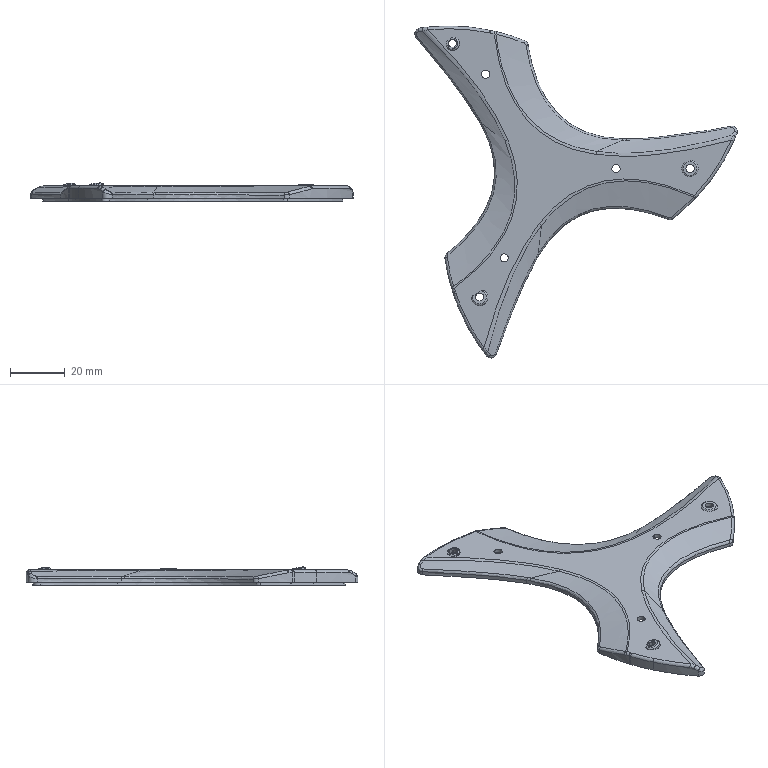Part | STEP file | ZXCOMPANY_A722-L-147 | 1 solid | 268 faces | box 117.864 x 121.275 x 6.608 mm | volume 9843 mm3 | spline 96 | cylinder 77 | other 35 | plane 31 | torus 20 | sphere 9 | commonest cylinder face diameters 3 x16 0.6 x7 1 x5 140.86 x5 143.86 x5 145.86 x5